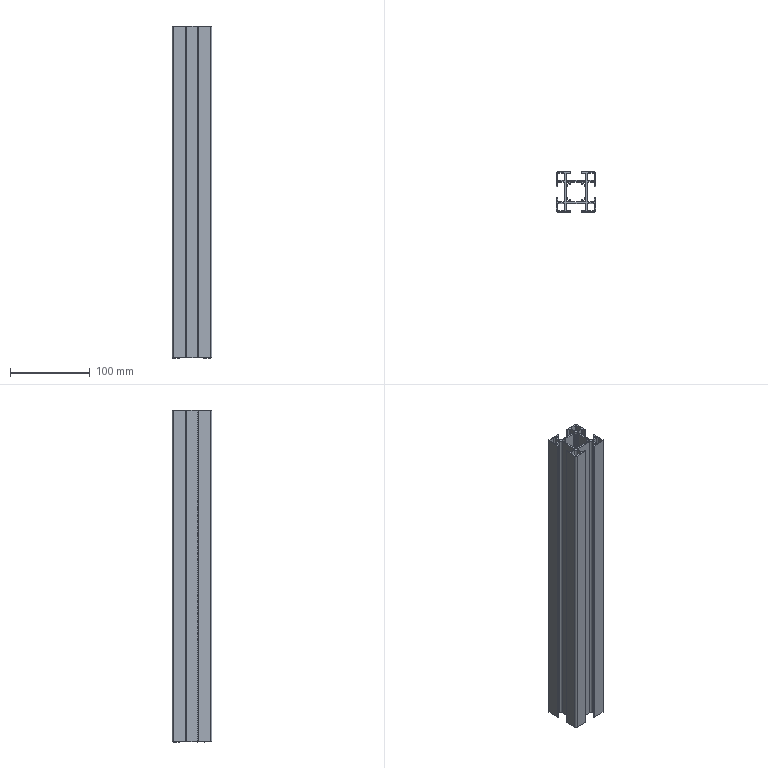Part | STEP file | 46A-00006CC11-417mm | 1 solid | 142 faces | box 50 x 50 x 417 mm | volume 244984 mm3 | cylinder 84 | plane 58 | commonest cylinder face diameters 1 x24 4 x24 1.5 x16 3.7 x8 6.7 x8 2 x4